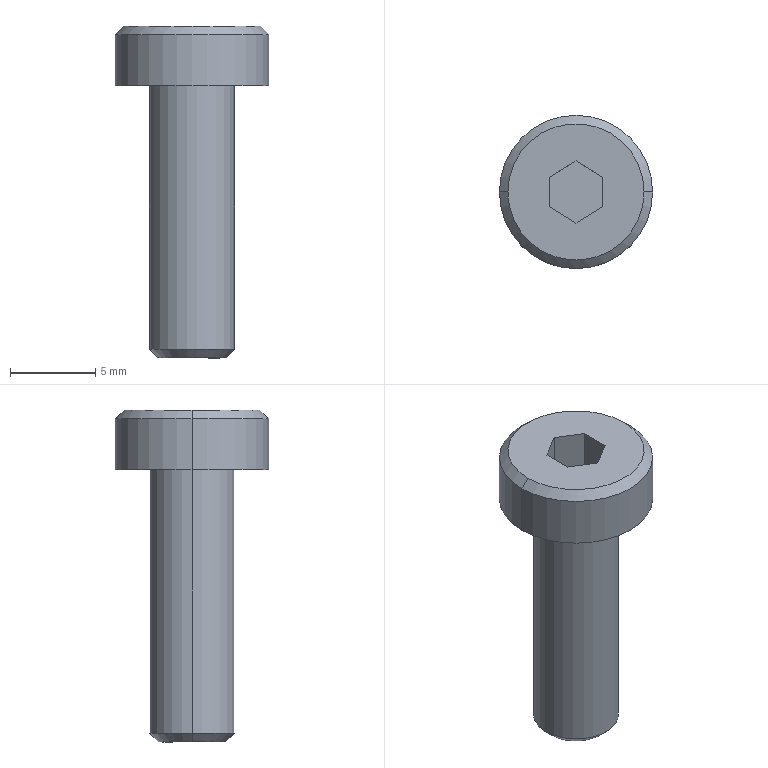Part | SolidWorks | features BaseBody 1 | 1 solid | 18 faces | box 9 x 9 x 19.5 mm | volume 507.431 mm3 | plane 10 | cone 4 | cylinder 4 | commonest cylinder face diameters 5 x2 9 x2
STEP:
#1=CARTESIAN_POINT('',(-10.,-21.,-14.816));
#2=VERTEX_POINT('',#1);
#3=CARTESIAN_POINT('',(-14.,-21.,-14.816));
#4=VERTEX_POINT('',#3);
#5=CARTESIAN_POINT('',(-12.,-21.,-14.816));
#6=DIRECTION('',(0.,0.,1.));
#7=DIRECTION('',(1.,0.,0.));
#8=AXIS2_PLACEMENT_3D('',#5,#6,#7);
#9=CIRCLE('',#8,2.);
#10=EDGE_CURVE('',#2,#4,#9,.T.);
#11=ORIENTED_EDGE('',*,*,#10,.F.);
#12=CARTESIAN_POINT('',(-12.,-21.,-14.816));
#13=DIRECTION('',(0.,0.,1.));
#14=DIRECTION('',(-1.,0.,0.));
#15=AXIS2_PLACEMENT_3D('',#12,#13,#14);
#16=CIRCLE('',#15,2.);
#17=EDGE_CURVE('',#4,#2,#16,.T.);
#18=ORIENTED_EDGE('',*,*,#17,.F.);
#19=EDGE_LOOP('',(#11,#18));
#20=FACE_OUTER_BOUND('',#19,.T.);
#21=CARTESIAN_POINT('',(-12.,-21.,-14.816));
#22=DIRECTION('',(0.,0.,-1.));
#23=DIRECTION('',(0.,-1.,0.));
#24=AXIS2_PLACEMENT_3D('',#21,#22,#23);
#25=PLANE('',#24);
#26=ADVANCED_FACE('',(#20),#25,.T.);
#27=ORIENTED_EDGE('',*,*,#17,.T.);
#28=CARTESIAN_POINT('',(-9.5,-21.,-14.316));
#29=VERTEX_POINT('',#28);
#30=CARTESIAN_POINT('',(-9.5,-21.,-14.316));
#31=DIRECTION('',(-0.7071,0.,-0.7071));
#32=VECTOR('',#31,1000.);
#33=LINE('',#30,#32);
#34=EDGE_CURVE('',#29,#2,#33,.T.);
#35=ORIENTED_EDGE('',*,*,#34,.F.);
#36=CARTESIAN_POINT('',(-14.5,-21.,-14.316));
#37=VERTEX_POINT('',#36);
#38=CARTESIAN_POINT('',(-12.,-21.,-14.316));
#39=DIRECTION('',(0.,0.,1.));
#40=DIRECTION('',(-1.,0.,0.));
#41=AXIS2_PLACEMENT_3D('',#38,#39,#40);
#42=CIRCLE('',#41,2.5);
#43=EDGE_CURVE('',#37,#29,#42,.T.);
#44=ORIENTED_EDGE('',*,*,#43,.F.);
#45=CARTESIAN_POINT('',(-14.5,-21.,-14.316));
#46=DIRECTION('',(0.7071,0.,-0.7071));
#47=VECTOR('',#46,1000.);
#48=LINE('',#45,#47);
#49=EDGE_CURVE('',#37,#4,#48,.T.);
#50=ORIENTED_EDGE('',*,*,#49,.T.);
#51=EDGE_LOOP('',(#27,#35,#44,#50));
#52=FACE_OUTER_BOUND('',#51,.T.);
#53=CARTESIAN_POINT('',(-12.,-21.,-14.566));
#54=DIRECTION('',(0.,0.,1.));
#55=DIRECTION('',(1.,0.,0.));
#56=AXIS2_PLACEMENT_3D('',#53,#54,#55);
#57=CONICAL_SURFACE('',#56,2.25,0.7854);
#58=ADVANCED_FACE('',(#52),#57,.T.);
#59=ORIENTED_EDGE('',*,*,#49,.F.);
#60=CARTESIAN_POINT('',(-12.,-21.,-14.316));
#61=DIRECTION('',(0.,0.,1.));
#62=DIRECTION('',(1.,0.,0.));
#63=AXIS2_PLACEMENT_3D('',#60,#61,#62);
#64=CIRCLE('',#63,2.5);
#65=EDGE_CURVE('',#29,#37,#64,.T.);
#66=ORIENTED_EDGE('',*,*,#65,.F.);
#67=ORIENTED_EDGE('',*,*,#34,.T.);
#68=ORIENTED_EDGE('',*,*,#10,.T.);
#69=EDGE_LOOP('',(#59,#66,#67,#68));
#70=FACE_OUTER_BOUND('',#69,.T.);
#71=CARTESIAN_POINT('',(-12.,-21.,-14.566));
#72=DIRECTION('',(0.,0.,1.));
#73=DIRECTION('',(1.,0.,0.));
#74=AXIS2_PLACEMENT_3D('',#71,#72,#73);
#75=CONICAL_SURFACE('',#74,2.25,0.7854);
#76=ADVANCED_FACE('',(#70),#75,.T.);
#77=CARTESIAN_POINT('',(-9.5,-21.,1.184));
#78=VERTEX_POINT('',#77);
#79=CARTESIAN_POINT('',(-9.5,-21.,-14.316));
#80=DIRECTION('',(0.,0.,1.));
#81=VECTOR('',#80,1000.);
#82=LINE('',#79,#81);
#83=EDGE_CURVE('',#29,#78,#82,.T.);
#84=ORIENTED_EDGE('',*,*,#83,.F.);
#85=ORIENTED_EDGE('',*,*,#65,.T.);
#86=CARTESIAN_POINT('',(-14.5,-21.,1.184));
#87=VERTEX_POINT('',#86);
#88=CARTESIAN_POINT('',(-14.5,-21.,-14.316));
#89=DIRECTION('',(0.,0.,1.));
#90=VECTOR('',#89,1000.);
#91=LINE('',#88,#90);
#92=EDGE_CURVE('',#37,#87,#91,.T.);
#93=ORIENTED_EDGE('',*,*,#92,.T.);
#94=CARTESIAN_POINT('',(-12.,-21.,1.184));
#95=DIRECTION('',(0.,0.,-1.));
#96=DIRECTION('',(-1.,0.,0.));
#97=AXIS2_PLACEMENT_3D('',#94,#95,#96);
#98=CIRCLE('',#97,2.5);
#99=EDGE_CURVE('',#87,#78,#98,.T.);
#100=ORIENTED_EDGE('',*,*,#99,.T.);
#101=EDGE_LOOP('',(#84,#85,#93,#100));
#102=FACE_OUTER_BOUND('',#101,.T.);
#103=CARTESIAN_POINT('',(-12.,-21.,1.184));
#104=DIRECTION('',(0.,0.,-1.));
#105=DIRECTION('',(-1.,0.,0.));
#106=AXIS2_PLACEMENT_3D('',#103,#104,#105);
#107=CYLINDRICAL_SURFACE('',#106,2.5);
#108=ADVANCED_FACE('',(#102),#107,.T.);
#109=CARTESIAN_POINT('',(-12.,-21.,1.184));
#110=DIRECTION('',(0.,0.,-1.));
#111=DIRECTION('',(1.,0.,0.));
#112=AXIS2_PLACEMENT_3D('',#109,#110,#111);
#113=CIRCLE('',#112,2.5);
#114=EDGE_CURVE('',#78,#87,#113,.T.);
#115=ORIENTED_EDGE('',*,*,#114,.F.);
#116=ORIENTED_EDGE('',*,*,#99,.F.);
#117=EDGE_LOOP('',(#115,#116));
#118=FACE_BOUND('',#117,.T.);
#119=CARTESIAN_POINT('',(-16.5,-21.,1.184));
#120=VERTEX_POINT('',#119);
#121=CARTESIAN_POINT('',(-7.5,-21.,1.184));
#122=VERTEX_POINT('',#121);
#123=CARTESIAN_POINT('',(-12.,-21.,1.184));
#124=DIRECTION('',(0.,0.,1.));
#125=DIRECTION('',(-1.,0.,0.));
#126=AXIS2_PLACEMENT_3D('',#123,#124,#125);
#127=CIRCLE('',#126,4.5);
#128=EDGE_CURVE('',#120,#122,#127,.T.);
#129=ORIENTED_EDGE('',*,*,#128,.F.);
#130=CARTESIAN_POINT('',(-12.,-21.,1.184));
#131=DIRECTION('',(0.,0.,1.));
#132=DIRECTION('',(1.,0.,0.));
#133=AXIS2_PLACEMENT_3D('',#130,#131,#132);
#134=CIRCLE('',#133,4.5);
#135=EDGE_CURVE('',#122,#120,#134,.T.);
#136=ORIENTED_EDGE('',*,*,#135,.F.);
#137=EDGE_LOOP('',(#129,#136));
#138=FACE_OUTER_BOUND('',#137,.T.);
#139=CARTESIAN_POINT('',(-12.,-21.,1.184));
#140=DIRECTION('',(0.,0.,-1.));
#141=DIRECTION('',(0.,-1.,0.));
#142=AXIS2_PLACEMENT_3D('',#139,#140,#141);
#143=PLANE('',#142);
#144=ADVANCED_FACE('',(#118,#138),#143,.T.);
#145=CARTESIAN_POINT('',(-7.5,-21.,4.184));
#146=VERTEX_POINT('',#145);
#147=CARTESIAN_POINT('',(-7.5,-21.,1.184));
#148=DIRECTION('',(0.,0.,1.));
#149=VECTOR('',#148,1000.);
#150=LINE('',#147,#149);
#151=EDGE_CURVE('',#122,#146,#150,.T.);
#152=ORIENTED_EDGE('',*,*,#151,.F.);
#153=ORIENTED_EDGE('',*,*,#135,.T.);
#154=CARTESIAN_POINT('',(-16.5,-21.,4.184));
#155=VERTEX_POINT('',#154);
#156=CARTESIAN_POINT('',(-16.5,-21.,1.184));
#157=DIRECTION('',(0.,0.,1.));
#158=VECTOR('',#157,1000.);
#159=LINE('',#156,#158);
#160=EDGE_CURVE('',#120,#155,#159,.T.);
#161=ORIENTED_EDGE('',*,*,#160,.T.);
#162=CARTESIAN_POINT('',(-12.,-21.,4.184));
#163=DIRECTION('',(0.,0.,-1.));
#164=DIRECTION('',(-1.,0.,0.));
#165=AXIS2_PLACEMENT_3D('',#162,#163,#164);
#166=CIRCLE('',#165,4.5);
#167=EDGE_CURVE('',#155,#146,#166,.T.);
#168=ORIENTED_EDGE('',*,*,#167,.T.);
#169=EDGE_LOOP('',(#152,#153,#161,#168));
#170=FACE_OUTER_BOUND('',#169,.T.);
#171=CARTESIAN_POINT('',(-12.,-21.,11.184));
#172=DIRECTION('',(0.,0.,-1.));
#173=DIRECTION('',(-1.,0.,0.));
#174=AXIS2_PLACEMENT_3D('',#171,#172,#173);
#175=CYLINDRICAL_SURFACE('',#174,4.5);
#176=ADVANCED_FACE('',(#170),#175,.T.);
#177=CARTESIAN_POINT('',(-8.,-21.,4.684));
#178=VERTEX_POINT('',#177);
#179=CARTESIAN_POINT('',(-7.5,-21.,4.184));
#180=DIRECTION('',(-0.7071,0.,0.7071));
#181=VECTOR('',#180,1000.);
#182=LINE('',#179,#181);
#183=EDGE_CURVE('',#146,#178,#182,.T.);
#184=ORIENTED_EDGE('',*,*,#183,.F.);
#185=ORIENTED_EDGE('',*,*,#167,.F.);
#186=CARTESIAN_POINT('',(-16.,-21.,4.684));
#187=VERTEX_POINT('',#186);
#188=CARTESIAN_POINT('',(-16.5,-21.,4.184));
#189=DIRECTION('',(0.7071,0.,0.7071));
#190=VECTOR('',#189,1000.);
#191=LINE('',#188,#190);
#192=EDGE_CURVE('',#155,#187,#191,.T.);
#193=ORIENTED_EDGE('',*,*,#192,.T.);
#194=CARTESIAN_POINT('',(-12.,-21.,4.684));
#195=DIRECTION('',(0.,0.,-1.));
#196=DIRECTION('',(-1.,0.,0.));
#197=AXIS2_PLACEMENT_3D('',#194,#195,#196);
#198=CIRCLE('',#197,4.);
#199=EDGE_CURVE('',#187,#178,#198,.T.);
#200=ORIENTED_EDGE('',*,*,#199,.T.);
#201=EDGE_LOOP('',(#184,#185,#193,#200));
#202=FACE_OUTER_BOUND('',#201,.T.);
#203=CARTESIAN_POINT('',(-12.,-21.,4.434));
#204=DIRECTION('',(0.,0.,-1.));
#205=DIRECTION('',(-1.,0.,0.));
#206=AXIS2_PLACEMENT_3D('',#203,#204,#205);
#207=CONICAL_SURFACE('',#206,4.25,0.7854);
#208=ADVANCED_FACE('',(#202),#207,.T.);
#209=CARTESIAN_POINT('',(-12.,-19.175,4.684));
#210=VERTEX_POINT('',#209);
#211=CARTESIAN_POINT('',(-10.45,-20.138,4.684));
#212=VERTEX_POINT('',#211);
#213=CARTESIAN_POINT('',(-12.,-19.175,4.684));
#214=DIRECTION('',(0.8494,-0.5278,0.));
#215=VECTOR('',#214,1000.);
#216=LINE('',#213,#215);
#217=EDGE_CURVE('',#210,#212,#216,.T.);
#218=ORIENTED_EDGE('',*,*,#217,.T.);
#219=CARTESIAN_POINT('',(-10.45,-21.862,4.684));
#220=VERTEX_POINT('',#219);
#221=CARTESIAN_POINT('',(-10.45,-20.138,4.684));
#222=DIRECTION('',(-0.000001796,-1.,0.));
#223=VECTOR('',#222,1000.);
#224=LINE('',#221,#223);
#225=EDGE_CURVE('',#212,#220,#224,.T.);
#226=ORIENTED_EDGE('',*,*,#225,.T.);
#227=CARTESIAN_POINT('',(-12.,-22.825,4.684));
#228=VERTEX_POINT('',#227);
#229=CARTESIAN_POINT('',(-10.45,-21.862,4.684));
#230=DIRECTION('',(-0.8494,-0.5278,0.));
#231=VECTOR('',#230,1000.);
#232=LINE('',#229,#231);
#233=EDGE_CURVE('',#220,#228,#232,.T.);
#234=ORIENTED_EDGE('',*,*,#233,.T.);
#235=CARTESIAN_POINT('',(-13.55,-21.862,4.684));
#236=VERTEX_POINT('',#235);
#237=CARTESIAN_POINT('',(-12.,-22.825,4.684));
#238=DIRECTION('',(-0.8494,0.5278,0.));
#239=VECTOR('',#238,1000.);
#240=LINE('',#237,#239);
#241=EDGE_CURVE('',#228,#236,#240,.T.);
#242=ORIENTED_EDGE('',*,*,#241,.T.);
#243=CARTESIAN_POINT('',(-13.55,-20.138,4.684));
#244=VERTEX_POINT('',#243);
#245=CARTESIAN_POINT('',(-13.55,-21.862,4.684));
#246=DIRECTION('',(0.000001977,1.,0.));
#247=VECTOR('',#246,1000.);
#248=LINE('',#245,#247);
#249=EDGE_CURVE('',#236,#244,#248,.T.);
#250=ORIENTED_EDGE('',*,*,#249,.T.);
#251=CARTESIAN_POINT('',(-13.55,-20.138,4.684));
#252=DIRECTION('',(0.8494,0.5278,0.));
#253=VECTOR('',#252,1000.);
#254=LINE('',#251,#253);
#255=EDGE_CURVE('',#244,#210,#254,.T.);
#256=ORIENTED_EDGE('',*,*,#255,.T.);
#257=EDGE_LOOP('',(#218,#226,#234,#242,#250,#256));
#258=FACE_BOUND('',#257,.T.);
#259=ORIENTED_EDGE('',*,*,#199,.F.);
#260=CARTESIAN_POINT('',(-12.,-21.,4.684));
#261=DIRECTION('',(0.,0.,-1.));
#262=DIRECTION('',(1.,0.,0.));
#263=AXIS2_PLACEMENT_3D('',#260,#261,#262);
#264=CIRCLE('',#263,4.);
#265=EDGE_CURVE('',#178,#187,#264,.T.);
#266=ORIENTED_EDGE('',*,*,#265,.F.);
#267=EDGE_LOOP('',(#259,#266));
#268=FACE_OUTER_BOUND('',#267,.T.);
#269=CARTESIAN_POINT('',(-12.,-21.,4.684));
#270=DIRECTION('',(0.,0.,1.));
#271=DIRECTION('',(1.,0.,0.));
#272=AXIS2_PLACEMENT_3D('',#269,#270,#271);
#273=PLANE('',#272);
#274=ADVANCED_FACE('',(#258,#268),#273,.T.);
#275=ORIENTED_EDGE('',*,*,#265,.T.);
#276=ORIENTED_EDGE('',*,*,#192,.F.);
#277=CARTESIAN_POINT('',(-12.,-21.,4.184));
#278=DIRECTION('',(0.,0.,-1.));
#279=DIRECTION('',(1.,0.,0.));
#280=AXIS2_PLACEMENT_3D('',#277,#278,#279);
#281=CIRCLE('',#280,4.5);
#282=EDGE_CURVE('',#146,#155,#281,.T.);
#283=ORIENTED_EDGE('',*,*,#282,.F.);
#284=ORIENTED_EDGE('',*,*,#183,.T.);
#285=EDGE_LOOP('',(#275,#276,#283,#284));
#286=FACE_OUTER_BOUND('',#285,.T.);
#287=CARTESIAN_POINT('',(-12.,-21.,4.434));
#288=DIRECTION('',(0.,0.,-1.));
#289=DIRECTION('',(-1.,0.,0.));
#290=AXIS2_PLACEMENT_3D('',#287,#288,#289);
#291=CONICAL_SURFACE('',#290,4.25,0.7854);
#292=ADVANCED_FACE('',(#286),#291,.T.);
#293=ORIENTED_EDGE('',*,*,#282,.T.);
#294=ORIENTED_EDGE('',*,*,#160,.F.);
#295=ORIENTED_EDGE('',*,*,#128,.T.);
#296=ORIENTED_EDGE('',*,*,#151,.T.);
#297=EDGE_LOOP('',(#293,#294,#295,#296));
#298=FACE_OUTER_BOUND('',#297,.T.);
#299=CARTESIAN_POINT('',(-12.,-21.,11.184));
#300=DIRECTION('',(0.,0.,-1.));
#301=DIRECTION('',(-1.,0.,0.));
#302=AXIS2_PLACEMENT_3D('',#299,#300,#301);
#303=CYLINDRICAL_SURFACE('',#302,4.5);
#304=ADVANCED_FACE('',(#298),#303,.T.);
#305=CARTESIAN_POINT('',(-12.,-19.175,1.784));
#306=VERTEX_POINT('',#305);
#307=CARTESIAN_POINT('',(-12.,-19.175,4.184));
#308=DIRECTION('',(0.,0.,1.));
#309=VECTOR('',#308,1000.);
#310=LINE('',#307,#309);
#311=EDGE_CURVE('',#306,#210,#310,.T.);
#312=ORIENTED_EDGE('',*,*,#311,.T.);
#313=ORIENTED_EDGE('',*,*,#255,.F.);
#314=CARTESIAN_POINT('',(-13.55,-20.138,1.784));
#315=VERTEX_POINT('',#314);
#316=CARTESIAN_POINT('',(-13.55,-20.138,1.784));
#317=DIRECTION('',(0.,0.,1.));
#318=VECTOR('',#317,1000.);
#319=LINE('',#316,#318);
#320=EDGE_CURVE('',#315,#244,#319,.T.);
#321=ORIENTED_EDGE('',*,*,#320,.F.);
#322=CARTESIAN_POINT('',(-13.55,-20.138,1.784));
#323=DIRECTION('',(0.8494,0.5278,0.));
#324=VECTOR('',#323,1000.);
#325=LINE('',#322,#324);
#326=EDGE_CURVE('',#315,#306,#325,.T.);
#327=ORIENTED_EDGE('',*,*,#326,.T.);
#328=EDGE_LOOP('',(#312,#313,#321,#327));
#329=FACE_OUTER_BOUND('',#328,.T.);
#330=CARTESIAN_POINT('',(-12.,-19.175,4.184));
#331=DIRECTION('',(-0.5278,0.8494,0.));
#332=DIRECTION('',(0.,0.,1.));
#333=AXIS2_PLACEMENT_3D('',#330,#331,#332);
#334=PLANE('',#333);
#335=ADVANCED_FACE('',(#329),#334,.F.);
#336=CARTESIAN_POINT('',(-10.45,-20.138,4.184));
#337=VERTEX_POINT('',#336);
#338=CARTESIAN_POINT('',(-10.45,-20.138,4.684));
#339=DIRECTION('',(0.000000343,-0.000000958,-1.));
#340=VECTOR('',#339,1000.);
#341=LINE('',#338,#340);
#342=EDGE_CURVE('',#212,#337,#341,.T.);
#343=ORIENTED_EDGE('',*,*,#342,.F.);
#344=ORIENTED_EDGE('',*,*,#217,.F.);
#345=ORIENTED_EDGE('',*,*,#311,.F.);
#346=CARTESIAN_POINT('',(-10.45,-20.138,1.784));
#347=VERTEX_POINT('',#346);
#348=CARTESIAN_POINT('',(-12.,-19.175,1.784));
#349=DIRECTION('',(0.8494,-0.5278,0.));
#350=VECTOR('',#349,1000.);
#351=LINE('',#348,#350);
#352=EDGE_CURVE('',#306,#347,#351,.T.);
#353=ORIENTED_EDGE('',*,*,#352,.T.);
#354=CARTESIAN_POINT('',(-10.45,-20.138,4.184));
#355=DIRECTION('',(0.000000059,-0.000000109,-1.));
#356=VECTOR('',#355,1000.);
#357=LINE('',#354,#356);
#358=EDGE_CURVE('',#337,#347,#357,.T.);
#359=ORIENTED_EDGE('',*,*,#358,.F.);
#360=EDGE_LOOP('',(#343,#344,#345,#353,#359));
#361=FACE_OUTER_BOUND('',#360,.T.);
#362=CARTESIAN_POINT('',(-10.45,-20.138,4.184));
#363=DIRECTION('',(0.5278,0.8494,0.));
#364=DIRECTION('',(0.,0.,-1.));
#365=AXIS2_PLACEMENT_3D('',#362,#363,#364);
#366=PLANE('',#365);
#367=ADVANCED_FACE('',(#361),#366,.F.);
#368=ORIENTED_EDGE('',*,*,#225,.F.);
#369=ORIENTED_EDGE('',*,*,#342,.T.);
#370=ORIENTED_EDGE('',*,*,#358,.T.);
#371=CARTESIAN_POINT('',(-10.45,-21.862,1.784));
#372=VERTEX_POINT('',#371);
#373=CARTESIAN_POINT('',(-10.45,-20.138,1.784));
#374=DIRECTION('',(-0.000001977,-1.,0.));
#375=VECTOR('',#374,1000.);
#376=LINE('',#373,#375);
#377=EDGE_CURVE('',#347,#372,#376,.T.);
#378=ORIENTED_EDGE('',*,*,#377,.T.);
#379=CARTESIAN_POINT('',(-10.45,-21.862,1.784));
#380=DIRECTION('',(0.,0.,1.));
#381=VECTOR('',#380,1000.);
#382=LINE('',#379,#381);
#383=EDGE_CURVE('',#372,#220,#382,.T.);
#384=ORIENTED_EDGE('',*,*,#383,.T.);
#385=EDGE_LOOP('',(#368,#369,#370,#378,#384));
#386=FACE_OUTER_BOUND('',#385,.T.);
#387=CARTESIAN_POINT('',(-10.45,-21.862,4.184));
#388=DIRECTION('',(1.,-0.000001977,0.));
#389=DIRECTION('',(0.,0.,-1.));
#390=AXIS2_PLACEMENT_3D('',#387,#388,#389);
#391=PLANE('',#390);
#392=ADVANCED_FACE('',(#386),#391,.F.);
#393=CARTESIAN_POINT('',(-12.,-22.825,1.784));
#394=VERTEX_POINT('',#393);
#395=CARTESIAN_POINT('',(-12.,-22.825,4.184));
#396=DIRECTION('',(0.,0.,1.));
#397=VECTOR('',#396,1000.);
#398=LINE('',#395,#397);
#399=EDGE_CURVE('',#394,#228,#398,.T.);
#400=ORIENTED_EDGE('',*,*,#399,.T.);
#401=ORIENTED_EDGE('',*,*,#233,.F.);
#402=ORIENTED_EDGE('',*,*,#383,.F.);
#403=CARTESIAN_POINT('',(-10.45,-21.862,1.784));
#404=DIRECTION('',(-0.8494,-0.5278,0.));
#405=VECTOR('',#404,1000.);
#406=LINE('',#403,#405);
#407=EDGE_CURVE('',#372,#394,#406,.T.);
#408=ORIENTED_EDGE('',*,*,#407,.T.);
#409=EDGE_LOOP('',(#400,#401,#402,#408));
#410=FACE_OUTER_BOUND('',#409,.T.);
#411=CARTESIAN_POINT('',(-12.,-22.825,4.184));
#412=DIRECTION('',(0.5278,-0.8494,0.));
#413=DIRECTION('',(0.,0.,-1.));
#414=AXIS2_PLACEMENT_3D('',#411,#412,#413);
#415=PLANE('',#414);
#416=ADVANCED_FACE('',(#410),#415,.F.);
#417=ORIENTED_EDGE('',*,*,#241,.F.);
#418=ORIENTED_EDGE('',*,*,#399,.F.);
#419=CARTESIAN_POINT('',(-13.55,-21.862,1.784));
#420=VERTEX_POINT('',#419);
#421=CARTESIAN_POINT('',(-12.,-22.825,1.784));
#422=DIRECTION('',(-0.8494,0.5278,0.));
#423=VECTOR('',#422,1000.);
#424=LINE('',#421,#423);
#425=EDGE_CURVE('',#394,#420,#424,.T.);
#426=ORIENTED_EDGE('',*,*,#425,.T.);
#427=CARTESIAN_POINT('',(-13.55,-21.862,4.684));
#428=DIRECTION('',(0.,0.,-1.));
#429=VECTOR('',#428,1000.);
#430=LINE('',#427,#429);
#431=EDGE_CURVE('',#236,#420,#430,.T.);
#432=ORIENTED_EDGE('',*,*,#431,.F.);
#433=EDGE_LOOP('',(#417,#418,#426,#432));
#434=FACE_OUTER_BOUND('',#433,.T.);
#435=CARTESIAN_POINT('',(-13.55,-21.862,4.184));
#436=DIRECTION('',(-0.5278,-0.8494,0.));
#437=DIRECTION('',(-0.8494,0.5278,0.));
#438=AXIS2_PLACEMENT_3D('',#435,#436,#437);
#439=PLANE('',#438);
#440=ADVANCED_FACE('',(#434),#439,.F.);
#441=ORIENTED_EDGE('',*,*,#249,.F.);
#442=ORIENTED_EDGE('',*,*,#431,.T.);
#443=CARTESIAN_POINT('',(-13.55,-21.862,1.784));
#444=DIRECTION('',(0.000001977,1.,0.));
#445=VECTOR('',#444,1000.);
#446=LINE('',#443,#445);
#447=EDGE_CURVE('',#420,#315,#446,.T.);
#448=ORIENTED_EDGE('',*,*,#447,.T.);
#449=ORIENTED_EDGE('',*,*,#320,.T.);
#450=EDGE_LOOP('',(#441,#442,#448,#449));
#451=FACE_OUTER_BOUND('',#450,.T.);
#452=CARTESIAN_POINT('',(-13.55,-20.138,4.184));
#453=DIRECTION('',(-1.,0.000001977,0.));
#454=DIRECTION('',(0.,0.,1.));
#455=AXIS2_PLACEMENT_3D('',#452,#453,#454);
#456=PLANE('',#455);
#457=ADVANCED_FACE('',(#451),#456,.F.);
#458=ORIENTED_EDGE('',*,*,#447,.F.);
#459=ORIENTED_EDGE('',*,*,#425,.F.);
#460=ORIENTED_EDGE('',*,*,#407,.F.);
#461=ORIENTED_EDGE('',*,*,#377,.F.);
#462=ORIENTED_EDGE('',*,*,#352,.F.);
#463=ORIENTED_EDGE('',*,*,#326,.F.);
#464=EDGE_LOOP('',(#458,#459,#460,#461,#462,#463));
#465=FACE_OUTER_BOUND('',#464,.T.);
#466=CARTESIAN_POINT('',(-12.,-21.,1.784));
#467=DIRECTION('',(0.,0.,1.));
#468=DIRECTION('',(1.,0.,0.));
#469=AXIS2_PLACEMENT_3D('',#466,#467,#468);
#470=PLANE('',#469);
#471=ADVANCED_FACE('',(#465),#470,.T.);
#472=ORIENTED_EDGE('',*,*,#114,.T.);
#473=ORIENTED_EDGE('',*,*,#92,.F.);
#474=ORIENTED_EDGE('',*,*,#43,.T.);
#475=ORIENTED_EDGE('',*,*,#83,.T.);
#476=EDGE_LOOP('',(#472,#473,#474,#475));
#477=FACE_OUTER_BOUND('',#476,.T.);
#478=CARTESIAN_POINT('',(-12.,-21.,1.184));
#479=DIRECTION('',(0.,0.,-1.));
#480=DIRECTION('',(-1.,0.,0.));
#481=AXIS2_PLACEMENT_3D('',#478,#479,#480);
#482=CYLINDRICAL_SURFACE('',#481,2.5);
#483=ADVANCED_FACE('',(#477),#482,.T.);
#484=CLOSED_SHELL('',(#26,#58,#76,#108,#144,#176,#208,#274,#292,#304,#335,#367,#392,#416,#440,#457,#471,#483));
#485=MANIFOLD_SOLID_BREP('',#484);
#486=CARTESIAN_POINT('',(0.,0.,0.));
#487=DIRECTION('',(0.,0.,1.));
#488=DIRECTION('',(1.,0.,0.));
#489=AXIS2_PLACEMENT_3D('',#486,#487,#488);
#490=(LENGTH_UNIT()NAMED_UNIT(*)SI_UNIT(.MILLI.,.METRE.));
#491=UNCERTAINTY_MEASURE_WITH_UNIT(LENGTH_MEASURE(0.00001),#490,'','');
#492=(NAMED_UNIT(*)PLANE_ANGLE_UNIT()SI_UNIT($,.RADIAN.));
#493=(NAMED_UNIT(*)SI_UNIT($,.STERADIAN.)SOLID_ANGLE_UNIT());
#494=(GEOMETRIC_REPRESENTATION_CONTEXT(3)GLOBAL_UNCERTAINTY_ASSIGNED_CONTEXT((#491))GLOBAL_UNIT_ASSIGNED_CONTEXT((#490,#492,#493))REPRESENTATION_CONTEXT('',''));
#495=ADVANCED_BREP_SHAPE_REPRESENTATION('',(#485,#489),#494);